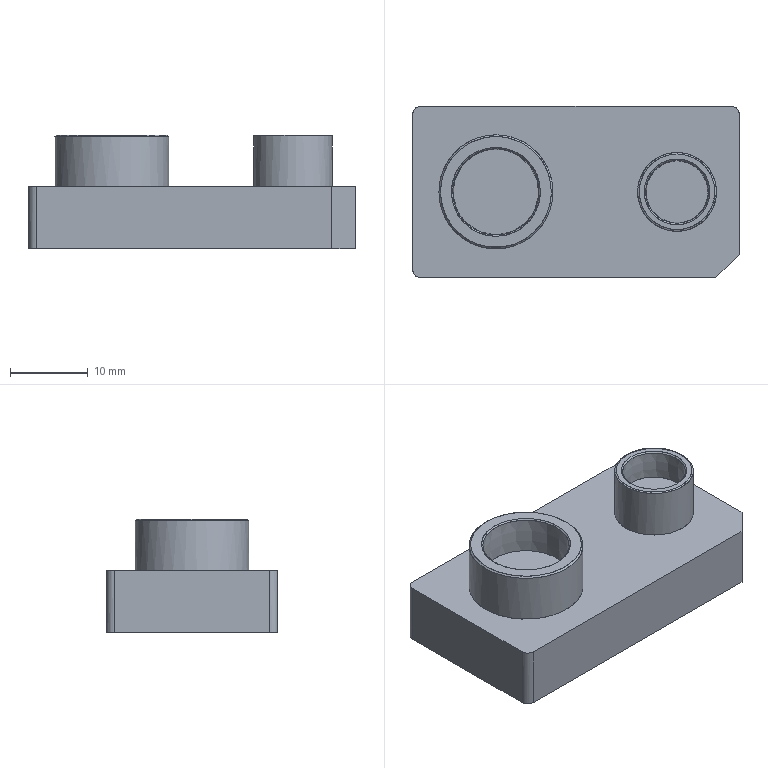CAM job | PowerMill | 3-axis milling, other | part box 42 x 22 x 14.621 mm
Tools:
number,name,type,diameter,tip_radius,length,cutting_length,overhang,flutes,holder,toolpaths_using
1,D10C,end_mill,10.0,0.0,60.0,,30.0,1,D42L35,1
14,D4_2,end_mill,4.0,0.0,30.0,,6.8,1,D42L35,2
1,D10C_1_1,end_mill,10.0,0.0,60.0,,15.08,1,D42L35,3
2,D4C_1_1,end_mill,4.0,0.0,30.0,,6.8,1,D42L35,1
3,D10_1_1,end_mill,10.0,0.0,60.0,,14.8,1,D42L35,3
13,Text_D4_1_1,taper_spherical,4.0,0.3,60.0,,6.88,1,D42L35,1
Operations:
program,toolpath,strategy,tool,tool_number,tool_diameter,tip_radius,flutes,spindle_rpm,feed_cut,surface_speed_m_min_computed,feed_per_tooth_computed,tolerance,thickness,stepover,stepdown,cut_length,cut_time_min,total_time_min,workplane
04-0318-1-F,精公开粗01-扫面平行-D10C,raster_area_clear,D10C_1_1,1,10.0,0.0,1.0,8000.0,10000.0,251.33,1.25,0.03,0.28,6.0,1.0,312.92,0.031,0.0376,
04-0318-1-F,精公开粗01-外形偏置-D10C,offset_area_clear,D10C_1_1,1,10.0,0.0,1.0,8000.0,10000.0,251.33,1.25,0.03,0.28,6.0,1.0,5290.534,0.529,0.574,
04-0318-1-F,精公开粗01-基准台等高-D10C,constantz,D10C_1_1,1,10.0,0.0,1.0,8000.0,10000.0,251.33,1.25,0.03,0.07,5.0,0.4,3449.063,0.345,0.3541,
04-0318-1-F,精公再粗02-外形偏置-D4C,offset_area_clear,D4C_1_1,2,4.0,0.0,1.0,18000.0,6000.0,226.19,0.3333,0.03,0.0,2.0,1.0,5217.407,0.87,1.163,
04-0318-1-F,精公基准台01-平坦面平行-D10,raster_area_clear,D10_1_1,3,10.0,0.0,1.0,8500.0,600.0,267.04,0.0706,0.005,0.38,5.0,1.0,215.959,0.36,0.3926,
04-0318-1-F,精公基准台01-基准面偏置-D10,offset_area_clear,D10_1_1,3,10.0,0.0,1.0,8500.0,600.0,267.04,0.0706,0.005,0.38,5.0,1.0,158.46,0.264,0.303,
04-0318-1-F,精公基准台01-基准台侧光-D10,profile_area_clear,D10_1_1,3,10.0,0.0,1.0,8500.0,600.0,267.04,0.0706,0.005,0.0,0.08,1.0,313.233,0.522,0.5858,
04-0318-1-F,精公精光01-等高-D4,constantz,D4_2,14,4.0,0.0,1.0,18000.0,2000.0,226.19,0.1111,0.005,-0.075,5.0,0.02,15047.928,7.524,8.19,
04-0318-1-F,精公精光01-平坦面偏置-D4,offset_area_clear,D4_2,14,4.0,0.0,1.0,18000.0,600.0,226.19,0.0333,0.005,0.375,2.0,1.0,226.899,0.378,0.4512,
04-0318-1-F,精公刻字01-刻字-Text_D4,pattern,Text_D4_1_1,13,4.0,0.3,1.0,15000.0,1000.0,188.5,0.0667,0.005,0.0,5.0,1.0,41.586,0.042,0.0591,
,精公开粗01-外形偏置-D10C_Reference,offset_area_clear,D10C,1,10.0,0.0,1.0,8000.0,10000.0,251.33,1.25,0.03,0.28,6.0,1.0,10269.63,1.027,1.111,